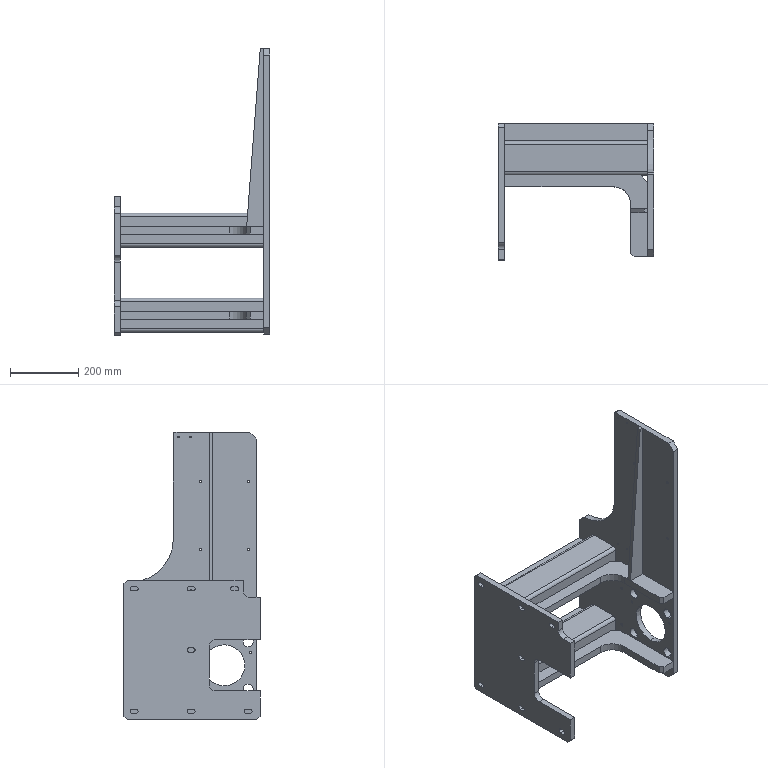Part | STEP file | PN_0002 Support seat 2_default_machined_ | 9 solids | 194 faces | box 457 x 400 x 845 mm | volume 11043445 mm3 | plane 99 | cylinder 89 | cone 6 | commonest cylinder face diameters 6.8 x24 13 x14 8.5 x11 5 x8 8 x8 20 x8